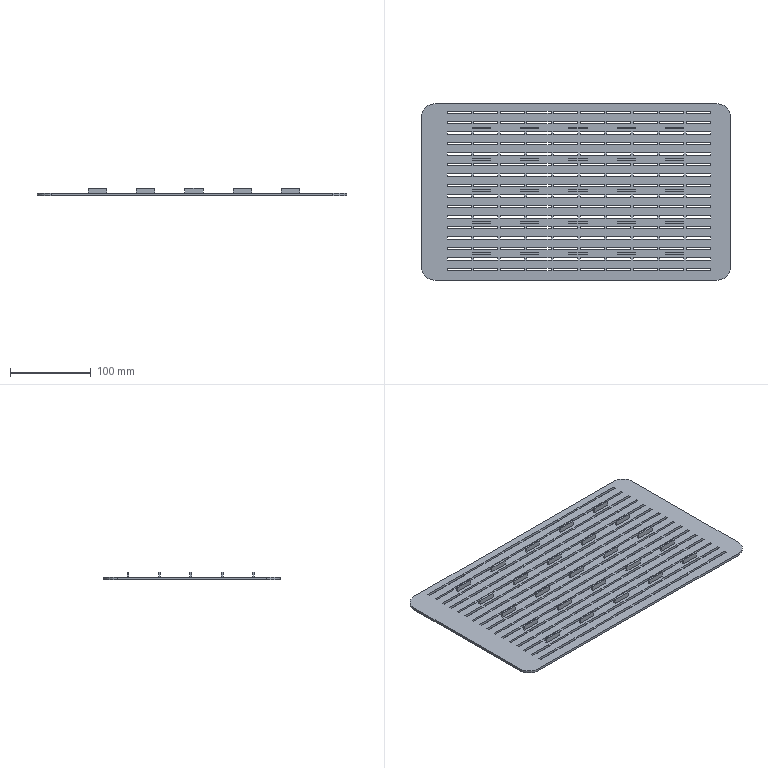Part | SolidWorks | features ICE 2, LPattern 2, Extrusion 1, Fillet 1 | 1 solid | 775 faces | box 384 x 219 x 9 mm | volume 215244 mm3 | plane 771 | cylinder 4 | commonest cylinder face diameters 34 x4